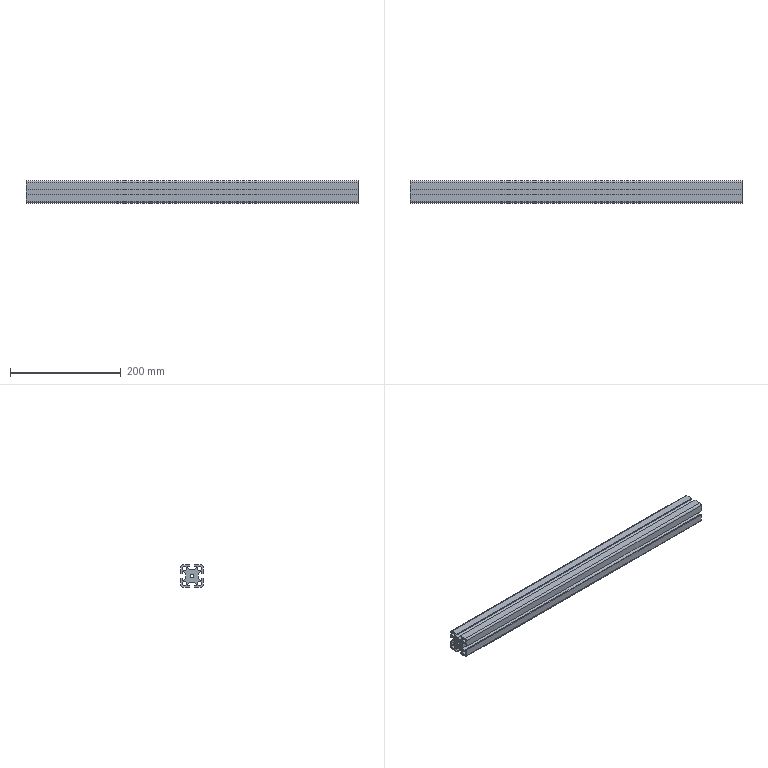Part | NX | 1 solid | 60 faces | box 600 x 40 x 40 mm | volume 536854 mm3 | plane 46 | cylinder 14 | commonest cylinder face diameters 8 x8 6.78 x4 6.8 x2